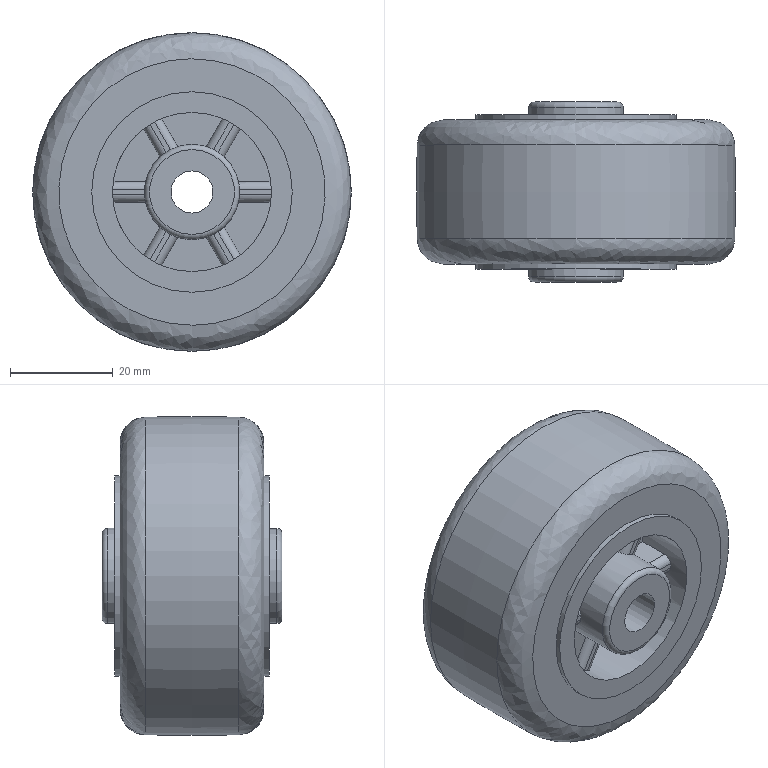Part | STEP file | 04FS0060~8.2.62.T35 | 1 solid | 90 faces | box 62 x 35 x 62 mm | volume 74583 mm3 | plane 54 | cylinder 31 | spline 2 | torus 2 | other 1 | commonest cylinder face diameters 3 x24 18.5 x2 31 x2 39 x2 8.2 x1